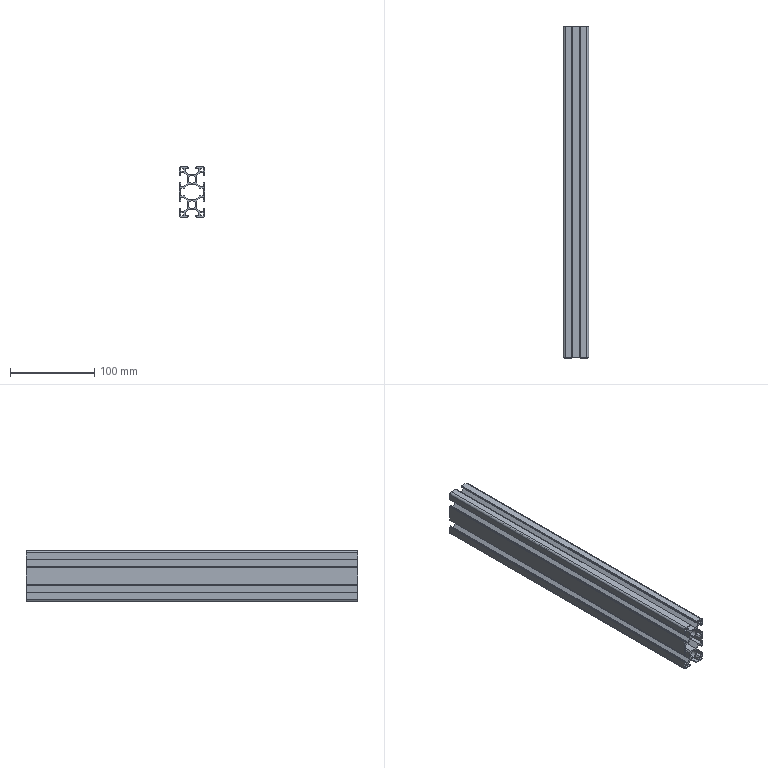Part | SolidWorks | features WeldMemberFeat 1, WeldmentFeature 1 | 1 solid | 126 faces | box 30 x 395 x 60 mm | volume 197620 mm3 | plane 118 | cylinder 8 | commonest cylinder face diameters 9.2 x4 3 x2 5 x2